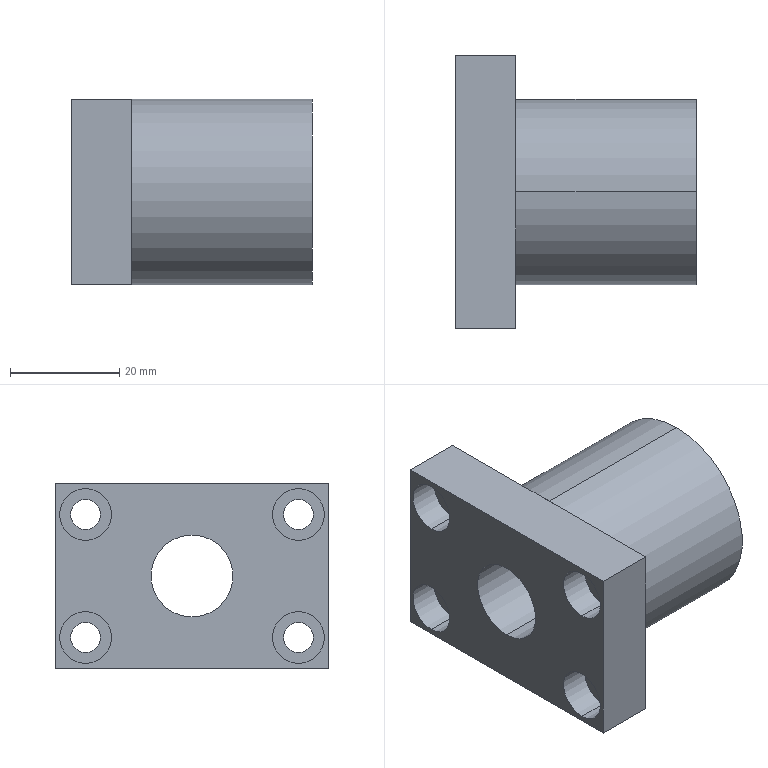Part | STEP file | Lead screw head | 1 solid | 32 faces | box 44 x 50 x 34 mm | volume 38804 mm3 | cylinder 20 | plane 12 | commonest cylinder face diameters 5.5 x8 9.5 x8 15 x2 34 x2